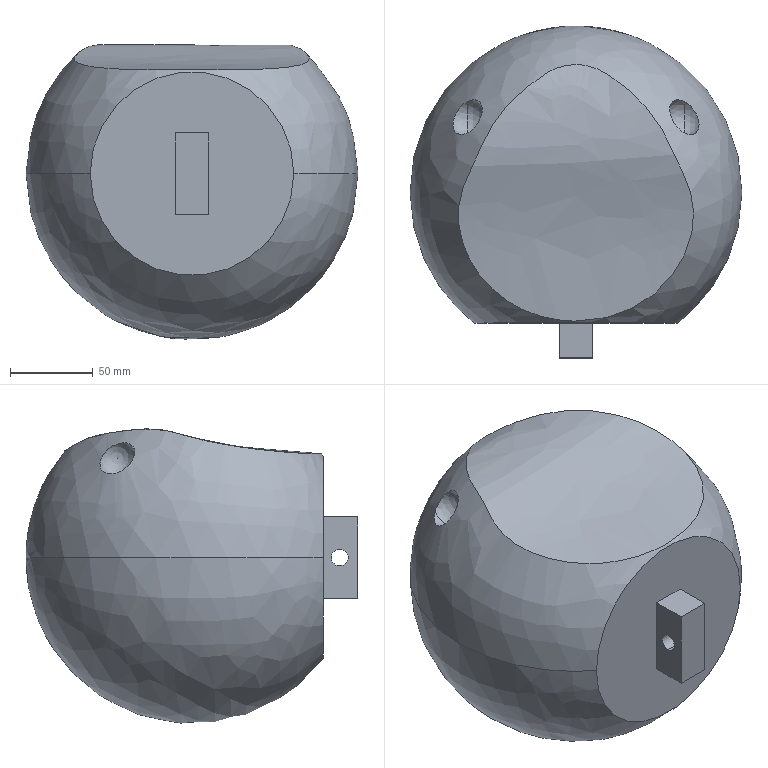Part | SolidWorks | features ICE 7, MirrorPattern 1, RevCut 1, Revolution 1 | 2 solids | 16 faces | volume 3831189 mm3 | plane 7 | sphere 4 | spline 3 | cylinder 2 | commonest cylinder face diameters 10.1 x2